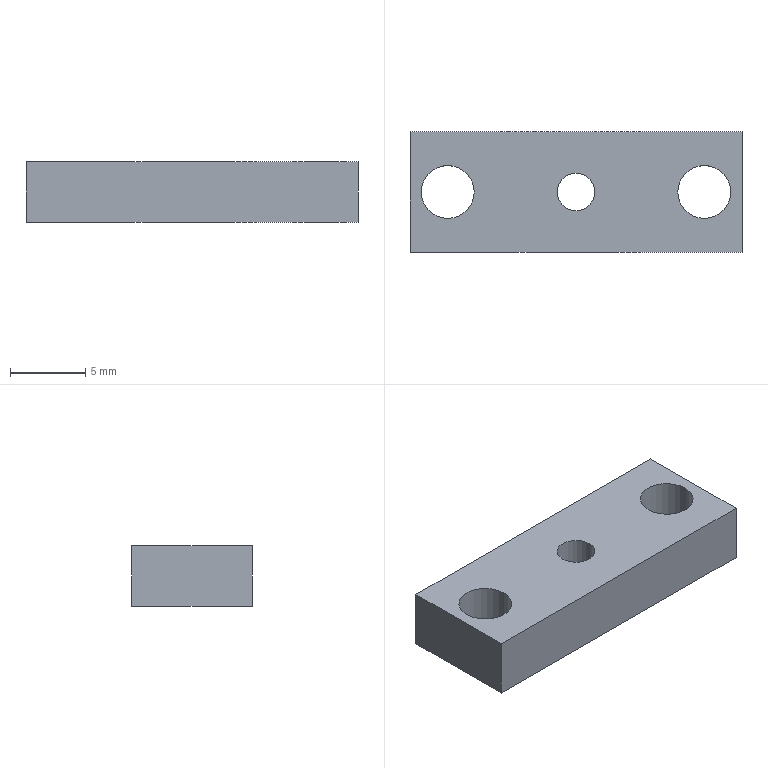Part | STEP file | X77b-01015 | 1 solid | 12 faces | box 22 x 8 x 4 mm | volume 607.396 mm3 | cylinder 6 | plane 6 | commonest cylinder face diameters 3.5 x4 2.5 x2
STEP:
#1=CARTESIAN_POINT('',(-1.25,-111.538,0.));
#2=VERTEX_POINT('',#1);
#3=CARTESIAN_POINT('',(1.25,-111.538,0.));
#4=VERTEX_POINT('',#3);
#5=CARTESIAN_POINT('',(0.,-111.538,0.));
#6=DIRECTION('',(0.,0.,1.));
#7=DIRECTION('',(1.,0.,0.));
#8=AXIS2_PLACEMENT_3D('',#5,#6,#7);
#9=CIRCLE('',#8,1.25);
#10=EDGE_CURVE('',#2,#4,#9,.T.);
#11=ORIENTED_EDGE('',*,*,#10,.F.);
#12=CARTESIAN_POINT('',(-1.25,-111.538,4.));
#13=VERTEX_POINT('',#12);
#14=CARTESIAN_POINT('',(-1.25,-111.538,4.));
#15=DIRECTION('',(0.,0.,1.));
#16=VECTOR('',#15,1000.);
#17=LINE('',#14,#16);
#18=EDGE_CURVE('',#2,#13,#17,.T.);
#19=ORIENTED_EDGE('',*,*,#18,.T.);
#20=CARTESIAN_POINT('',(1.25,-111.538,4.));
#21=VERTEX_POINT('',#20);
#22=CARTESIAN_POINT('',(0.,-111.538,4.));
#23=DIRECTION('',(0.,0.,1.));
#24=DIRECTION('',(1.,0.,0.));
#25=AXIS2_PLACEMENT_3D('',#22,#23,#24);
#26=CIRCLE('',#25,1.25);
#27=EDGE_CURVE('',#13,#21,#26,.T.);
#28=ORIENTED_EDGE('',*,*,#27,.T.);
#29=CARTESIAN_POINT('',(1.25,-111.538,4.));
#30=DIRECTION('',(0.,0.,1.));
#31=VECTOR('',#30,1000.);
#32=LINE('',#29,#31);
#33=EDGE_CURVE('',#4,#21,#32,.T.);
#34=ORIENTED_EDGE('',*,*,#33,.F.);
#35=EDGE_LOOP('',(#11,#19,#28,#34));
#36=FACE_OUTER_BOUND('',#35,.T.);
#37=CARTESIAN_POINT('',(0.,-111.538,4.));
#38=DIRECTION('',(0.,0.,1.));
#39=DIRECTION('',(1.,0.,0.));
#40=AXIS2_PLACEMENT_3D('',#37,#38,#39);
#41=CYLINDRICAL_SURFACE('',#40,1.25);
#42=ADVANCED_FACE('',(#36),#41,.F.);
#43=CARTESIAN_POINT('',(6.75,-111.538,4.));
#44=VERTEX_POINT('',#43);
#45=CARTESIAN_POINT('',(10.25,-111.538,4.));
#46=VERTEX_POINT('',#45);
#47=CARTESIAN_POINT('',(8.5,-111.538,4.));
#48=DIRECTION('',(0.,0.,1.));
#49=DIRECTION('',(1.,0.,0.));
#50=AXIS2_PLACEMENT_3D('',#47,#48,#49);
#51=CIRCLE('',#50,1.75);
#52=EDGE_CURVE('',#44,#46,#51,.T.);
#53=ORIENTED_EDGE('',*,*,#52,.T.);
#54=CARTESIAN_POINT('',(10.25,-111.538,0.));
#55=VERTEX_POINT('',#54);
#56=CARTESIAN_POINT('',(10.25,-111.538,4.));
#57=DIRECTION('',(0.,0.,-1.));
#58=VECTOR('',#57,1000.);
#59=LINE('',#56,#58);
#60=EDGE_CURVE('',#46,#55,#59,.T.);
#61=ORIENTED_EDGE('',*,*,#60,.T.);
#62=CARTESIAN_POINT('',(6.75,-111.538,0.));
#63=VERTEX_POINT('',#62);
#64=CARTESIAN_POINT('',(8.5,-111.538,0.));
#65=DIRECTION('',(0.,0.,1.));
#66=DIRECTION('',(1.,0.,0.));
#67=AXIS2_PLACEMENT_3D('',#64,#65,#66);
#68=CIRCLE('',#67,1.75);
#69=EDGE_CURVE('',#63,#55,#68,.T.);
#70=ORIENTED_EDGE('',*,*,#69,.F.);
#71=CARTESIAN_POINT('',(6.75,-111.538,4.));
#72=DIRECTION('',(0.,0.,-1.));
#73=VECTOR('',#72,1000.);
#74=LINE('',#71,#73);
#75=EDGE_CURVE('',#44,#63,#74,.T.);
#76=ORIENTED_EDGE('',*,*,#75,.F.);
#77=EDGE_LOOP('',(#53,#61,#70,#76));
#78=FACE_OUTER_BOUND('',#77,.T.);
#79=CARTESIAN_POINT('',(8.5,-111.538,4.));
#80=DIRECTION('',(0.,0.,-1.));
#81=DIRECTION('',(-1.,0.,0.));
#82=AXIS2_PLACEMENT_3D('',#79,#80,#81);
#83=CYLINDRICAL_SURFACE('',#82,1.75);
#84=ADVANCED_FACE('',(#78),#83,.F.);
#85=CARTESIAN_POINT('',(-10.25,-111.538,4.));
#86=VERTEX_POINT('',#85);
#87=CARTESIAN_POINT('',(-6.75,-111.538,4.));
#88=VERTEX_POINT('',#87);
#89=CARTESIAN_POINT('',(-8.5,-111.538,4.));
#90=DIRECTION('',(0.,0.,1.));
#91=DIRECTION('',(1.,0.,0.));
#92=AXIS2_PLACEMENT_3D('',#89,#90,#91);
#93=CIRCLE('',#92,1.75);
#94=EDGE_CURVE('',#86,#88,#93,.T.);
#95=ORIENTED_EDGE('',*,*,#94,.T.);
#96=CARTESIAN_POINT('',(-6.75,-111.538,0.));
#97=VERTEX_POINT('',#96);
#98=CARTESIAN_POINT('',(-6.75,-111.538,4.));
#99=DIRECTION('',(0.,0.,-1.));
#100=VECTOR('',#99,1000.);
#101=LINE('',#98,#100);
#102=EDGE_CURVE('',#88,#97,#101,.T.);
#103=ORIENTED_EDGE('',*,*,#102,.T.);
#104=CARTESIAN_POINT('',(-10.25,-111.538,0.));
#105=VERTEX_POINT('',#104);
#106=CARTESIAN_POINT('',(-8.5,-111.538,0.));
#107=DIRECTION('',(0.,0.,1.));
#108=DIRECTION('',(1.,0.,0.));
#109=AXIS2_PLACEMENT_3D('',#106,#107,#108);
#110=CIRCLE('',#109,1.75);
#111=EDGE_CURVE('',#105,#97,#110,.T.);
#112=ORIENTED_EDGE('',*,*,#111,.F.);
#113=CARTESIAN_POINT('',(-10.25,-111.538,4.));
#114=DIRECTION('',(0.,0.,-1.));
#115=VECTOR('',#114,1000.);
#116=LINE('',#113,#115);
#117=EDGE_CURVE('',#86,#105,#116,.T.);
#118=ORIENTED_EDGE('',*,*,#117,.F.);
#119=EDGE_LOOP('',(#95,#103,#112,#118));
#120=FACE_OUTER_BOUND('',#119,.T.);
#121=CARTESIAN_POINT('',(-8.5,-111.538,4.));
#122=DIRECTION('',(0.,0.,-1.));
#123=DIRECTION('',(-1.,0.,0.));
#124=AXIS2_PLACEMENT_3D('',#121,#122,#123);
#125=CYLINDRICAL_SURFACE('',#124,1.75);
#126=ADVANCED_FACE('',(#120),#125,.F.);
#127=CARTESIAN_POINT('',(0.,-111.538,4.));
#128=DIRECTION('',(0.,0.,1.));
#129=DIRECTION('',(1.,0.,0.));
#130=AXIS2_PLACEMENT_3D('',#127,#128,#129);
#131=CIRCLE('',#130,1.25);
#132=EDGE_CURVE('',#21,#13,#131,.T.);
#133=ORIENTED_EDGE('',*,*,#132,.F.);
#134=ORIENTED_EDGE('',*,*,#27,.F.);
#135=EDGE_LOOP('',(#133,#134));
#136=FACE_BOUND('',#135,.T.);
#137=ORIENTED_EDGE('',*,*,#94,.F.);
#138=CARTESIAN_POINT('',(-8.5,-111.538,4.));
#139=DIRECTION('',(0.,0.,1.));
#140=DIRECTION('',(1.,0.,0.));
#141=AXIS2_PLACEMENT_3D('',#138,#139,#140);
#142=CIRCLE('',#141,1.75);
#143=EDGE_CURVE('',#88,#86,#142,.T.);
#144=ORIENTED_EDGE('',*,*,#143,.F.);
#145=EDGE_LOOP('',(#137,#144));
#146=FACE_BOUND('',#145,.T.);
#147=CARTESIAN_POINT('',(-11.,-107.538,4.));
#148=VERTEX_POINT('',#147);
#149=CARTESIAN_POINT('',(-11.,-115.538,4.));
#150=VERTEX_POINT('',#149);
#151=CARTESIAN_POINT('',(-11.,-107.538,4.));
#152=DIRECTION('',(0.,-1.,0.));
#153=VECTOR('',#152,1000.);
#154=LINE('',#151,#153);
#155=EDGE_CURVE('',#148,#150,#154,.T.);
#156=ORIENTED_EDGE('',*,*,#155,.T.);
#157=CARTESIAN_POINT('',(11.,-115.538,4.));
#158=VERTEX_POINT('',#157);
#159=CARTESIAN_POINT('',(-11.,-115.538,4.));
#160=DIRECTION('',(1.,0.,0.));
#161=VECTOR('',#160,1000.);
#162=LINE('',#159,#161);
#163=EDGE_CURVE('',#150,#158,#162,.T.);
#164=ORIENTED_EDGE('',*,*,#163,.T.);
#165=CARTESIAN_POINT('',(11.,-107.538,4.));
#166=VERTEX_POINT('',#165);
#167=CARTESIAN_POINT('',(11.,-107.538,4.));
#168=DIRECTION('',(0.,1.,0.));
#169=VECTOR('',#168,1000.);
#170=LINE('',#167,#169);
#171=EDGE_CURVE('',#158,#166,#170,.T.);
#172=ORIENTED_EDGE('',*,*,#171,.T.);
#173=CARTESIAN_POINT('',(-11.,-107.538,4.));
#174=DIRECTION('',(-1.,0.,0.));
#175=VECTOR('',#174,1000.);
#176=LINE('',#173,#175);
#177=EDGE_CURVE('',#166,#148,#176,.T.);
#178=ORIENTED_EDGE('',*,*,#177,.T.);
#179=EDGE_LOOP('',(#156,#164,#172,#178));
#180=FACE_OUTER_BOUND('',#179,.T.);
#181=ORIENTED_EDGE('',*,*,#52,.F.);
#182=CARTESIAN_POINT('',(8.5,-111.538,4.));
#183=DIRECTION('',(0.,0.,1.));
#184=DIRECTION('',(1.,0.,0.));
#185=AXIS2_PLACEMENT_3D('',#182,#183,#184);
#186=CIRCLE('',#185,1.75);
#187=EDGE_CURVE('',#46,#44,#186,.T.);
#188=ORIENTED_EDGE('',*,*,#187,.F.);
#189=EDGE_LOOP('',(#181,#188));
#190=FACE_BOUND('',#189,.T.);
#191=CARTESIAN_POINT('',(-11.,-115.538,4.));
#192=DIRECTION('',(0.,0.,1.));
#193=DIRECTION('',(1.,0.,0.));
#194=AXIS2_PLACEMENT_3D('',#191,#192,#193);
#195=PLANE('',#194);
#196=ADVANCED_FACE('',(#136,#146,#180,#190),#195,.T.);
#197=CARTESIAN_POINT('',(0.,-111.538,0.));
#198=DIRECTION('',(0.,0.,1.));
#199=DIRECTION('',(1.,0.,0.));
#200=AXIS2_PLACEMENT_3D('',#197,#198,#199);
#201=CIRCLE('',#200,1.25);
#202=EDGE_CURVE('',#4,#2,#201,.T.);
#203=ORIENTED_EDGE('',*,*,#202,.T.);
#204=ORIENTED_EDGE('',*,*,#10,.T.);
#205=EDGE_LOOP('',(#203,#204));
#206=FACE_BOUND('',#205,.T.);
#207=ORIENTED_EDGE('',*,*,#111,.T.);
#208=CARTESIAN_POINT('',(-8.5,-111.538,0.));
#209=DIRECTION('',(0.,0.,1.));
#210=DIRECTION('',(1.,0.,0.));
#211=AXIS2_PLACEMENT_3D('',#208,#209,#210);
#212=CIRCLE('',#211,1.75);
#213=EDGE_CURVE('',#97,#105,#212,.T.);
#214=ORIENTED_EDGE('',*,*,#213,.T.);
#215=EDGE_LOOP('',(#207,#214));
#216=FACE_BOUND('',#215,.T.);
#217=CARTESIAN_POINT('',(-11.,-107.538,0.));
#218=VERTEX_POINT('',#217);
#219=CARTESIAN_POINT('',(-11.,-115.538,0.));
#220=VERTEX_POINT('',#219);
#221=CARTESIAN_POINT('',(-11.,-107.538,0.));
#222=DIRECTION('',(0.,-1.,0.));
#223=VECTOR('',#222,1000.);
#224=LINE('',#221,#223);
#225=EDGE_CURVE('',#218,#220,#224,.T.);
#226=ORIENTED_EDGE('',*,*,#225,.F.);
#227=CARTESIAN_POINT('',(11.,-107.538,0.));
#228=VERTEX_POINT('',#227);
#229=CARTESIAN_POINT('',(-11.,-107.538,0.));
#230=DIRECTION('',(-1.,0.,0.));
#231=VECTOR('',#230,1000.);
#232=LINE('',#229,#231);
#233=EDGE_CURVE('',#228,#218,#232,.T.);
#234=ORIENTED_EDGE('',*,*,#233,.F.);
#235=CARTESIAN_POINT('',(11.,-115.538,0.));
#236=VERTEX_POINT('',#235);
#237=CARTESIAN_POINT('',(11.,-107.538,0.));
#238=DIRECTION('',(0.,1.,0.));
#239=VECTOR('',#238,1000.);
#240=LINE('',#237,#239);
#241=EDGE_CURVE('',#236,#228,#240,.T.);
#242=ORIENTED_EDGE('',*,*,#241,.F.);
#243=CARTESIAN_POINT('',(-11.,-115.538,0.));
#244=DIRECTION('',(1.,0.,0.));
#245=VECTOR('',#244,1000.);
#246=LINE('',#243,#245);
#247=EDGE_CURVE('',#220,#236,#246,.T.);
#248=ORIENTED_EDGE('',*,*,#247,.F.);
#249=EDGE_LOOP('',(#226,#234,#242,#248));
#250=FACE_OUTER_BOUND('',#249,.T.);
#251=ORIENTED_EDGE('',*,*,#69,.T.);
#252=CARTESIAN_POINT('',(8.5,-111.538,0.));
#253=DIRECTION('',(0.,0.,1.));
#254=DIRECTION('',(1.,0.,0.));
#255=AXIS2_PLACEMENT_3D('',#252,#253,#254);
#256=CIRCLE('',#255,1.75);
#257=EDGE_CURVE('',#55,#63,#256,.T.);
#258=ORIENTED_EDGE('',*,*,#257,.T.);
#259=EDGE_LOOP('',(#251,#258));
#260=FACE_BOUND('',#259,.T.);
#261=CARTESIAN_POINT('',(-11.,-115.538,0.));
#262=DIRECTION('',(0.,0.,1.));
#263=DIRECTION('',(1.,0.,0.));
#264=AXIS2_PLACEMENT_3D('',#261,#262,#263);
#265=PLANE('',#264);
#266=ADVANCED_FACE('',(#206,#216,#250,#260),#265,.F.);
#267=ORIENTED_EDGE('',*,*,#225,.T.);
#268=CARTESIAN_POINT('',(-11.,-115.538,4.));
#269=DIRECTION('',(0.,0.,-1.));
#270=VECTOR('',#269,1000.);
#271=LINE('',#268,#270);
#272=EDGE_CURVE('',#150,#220,#271,.T.);
#273=ORIENTED_EDGE('',*,*,#272,.F.);
#274=ORIENTED_EDGE('',*,*,#155,.F.);
#275=CARTESIAN_POINT('',(-11.,-107.538,4.));
#276=DIRECTION('',(0.,0.,-1.));
#277=VECTOR('',#276,1000.);
#278=LINE('',#275,#277);
#279=EDGE_CURVE('',#148,#218,#278,.T.);
#280=ORIENTED_EDGE('',*,*,#279,.T.);
#281=EDGE_LOOP('',(#267,#273,#274,#280));
#282=FACE_OUTER_BOUND('',#281,.T.);
#283=CARTESIAN_POINT('',(-11.,-107.538,4.));
#284=DIRECTION('',(1.,0.,0.));
#285=DIRECTION('',(0.,1.,0.));
#286=AXIS2_PLACEMENT_3D('',#283,#284,#285);
#287=PLANE('',#286);
#288=ADVANCED_FACE('',(#282),#287,.F.);
#289=ORIENTED_EDGE('',*,*,#247,.T.);
#290=CARTESIAN_POINT('',(11.,-115.538,4.));
#291=DIRECTION('',(0.,0.,-1.));
#292=VECTOR('',#291,1000.);
#293=LINE('',#290,#292);
#294=EDGE_CURVE('',#158,#236,#293,.T.);
#295=ORIENTED_EDGE('',*,*,#294,.F.);
#296=ORIENTED_EDGE('',*,*,#163,.F.);
#297=ORIENTED_EDGE('',*,*,#272,.T.);
#298=EDGE_LOOP('',(#289,#295,#296,#297));
#299=FACE_OUTER_BOUND('',#298,.T.);
#300=CARTESIAN_POINT('',(-11.,-115.538,4.));
#301=DIRECTION('',(0.,1.,0.));
#302=DIRECTION('',(0.,0.,1.));
#303=AXIS2_PLACEMENT_3D('',#300,#301,#302);
#304=PLANE('',#303);
#305=ADVANCED_FACE('',(#299),#304,.F.);
#306=ORIENTED_EDGE('',*,*,#241,.T.);
#307=CARTESIAN_POINT('',(11.,-107.538,4.));
#308=DIRECTION('',(0.,0.,-1.));
#309=VECTOR('',#308,1000.);
#310=LINE('',#307,#309);
#311=EDGE_CURVE('',#166,#228,#310,.T.);
#312=ORIENTED_EDGE('',*,*,#311,.F.);
#313=ORIENTED_EDGE('',*,*,#171,.F.);
#314=ORIENTED_EDGE('',*,*,#294,.T.);
#315=EDGE_LOOP('',(#306,#312,#313,#314));
#316=FACE_OUTER_BOUND('',#315,.T.);
#317=CARTESIAN_POINT('',(11.,-107.538,4.));
#318=DIRECTION('',(-1.,0.,0.));
#319=DIRECTION('',(0.,-1.,0.));
#320=AXIS2_PLACEMENT_3D('',#317,#318,#319);
#321=PLANE('',#320);
#322=ADVANCED_FACE('',(#316),#321,.F.);
#323=ORIENTED_EDGE('',*,*,#233,.T.);
#324=ORIENTED_EDGE('',*,*,#279,.F.);
#325=ORIENTED_EDGE('',*,*,#177,.F.);
#326=ORIENTED_EDGE('',*,*,#311,.T.);
#327=EDGE_LOOP('',(#323,#324,#325,#326));
#328=FACE_OUTER_BOUND('',#327,.T.);
#329=CARTESIAN_POINT('',(-11.,-107.538,4.));
#330=DIRECTION('',(0.,-1.,0.));
#331=DIRECTION('',(0.,0.,-1.));
#332=AXIS2_PLACEMENT_3D('',#329,#330,#331);
#333=PLANE('',#332);
#334=ADVANCED_FACE('',(#328),#333,.F.);
#335=ORIENTED_EDGE('',*,*,#102,.F.);
#336=ORIENTED_EDGE('',*,*,#143,.T.);
#337=ORIENTED_EDGE('',*,*,#117,.T.);
#338=ORIENTED_EDGE('',*,*,#213,.F.);
#339=EDGE_LOOP('',(#335,#336,#337,#338));
#340=FACE_OUTER_BOUND('',#339,.T.);
#341=CARTESIAN_POINT('',(-8.5,-111.538,4.));
#342=DIRECTION('',(0.,0.,-1.));
#343=DIRECTION('',(-1.,0.,0.));
#344=AXIS2_PLACEMENT_3D('',#341,#342,#343);
#345=CYLINDRICAL_SURFACE('',#344,1.75);
#346=ADVANCED_FACE('',(#340),#345,.F.);
#347=ORIENTED_EDGE('',*,*,#60,.F.);
#348=ORIENTED_EDGE('',*,*,#187,.T.);
#349=ORIENTED_EDGE('',*,*,#75,.T.);
#350=ORIENTED_EDGE('',*,*,#257,.F.);
#351=EDGE_LOOP('',(#347,#348,#349,#350));
#352=FACE_OUTER_BOUND('',#351,.T.);
#353=CARTESIAN_POINT('',(8.5,-111.538,4.));
#354=DIRECTION('',(0.,0.,-1.));
#355=DIRECTION('',(-1.,0.,0.));
#356=AXIS2_PLACEMENT_3D('',#353,#354,#355);
#357=CYLINDRICAL_SURFACE('',#356,1.75);
#358=ADVANCED_FACE('',(#352),#357,.F.);
#359=ORIENTED_EDGE('',*,*,#18,.F.);
#360=ORIENTED_EDGE('',*,*,#202,.F.);
#361=ORIENTED_EDGE('',*,*,#33,.T.);
#362=ORIENTED_EDGE('',*,*,#132,.T.);
#363=EDGE_LOOP('',(#359,#360,#361,#362));
#364=FACE_OUTER_BOUND('',#363,.T.);
#365=CARTESIAN_POINT('',(0.,-111.538,4.));
#366=DIRECTION('',(0.,0.,1.));
#367=DIRECTION('',(1.,0.,0.));
#368=AXIS2_PLACEMENT_3D('',#365,#366,#367);
#369=CYLINDRICAL_SURFACE('',#368,1.25);
#370=ADVANCED_FACE('',(#364),#369,.F.);
#371=CLOSED_SHELL('',(#42,#84,#126,#196,#266,#288,#305,#322,#334,#346,#358,#370));
#372=MANIFOLD_SOLID_BREP('',#371);
#373=CARTESIAN_POINT('',(0.,0.,0.));
#374=DIRECTION('',(0.,0.,1.));
#375=DIRECTION('',(1.,0.,0.));
#376=AXIS2_PLACEMENT_3D('',#373,#374,#375);
#377=(LENGTH_UNIT()NAMED_UNIT(*)SI_UNIT(.MILLI.,.METRE.));
#378=UNCERTAINTY_MEASURE_WITH_UNIT(LENGTH_MEASURE(0.00001),#377,'','');
#379=(NAMED_UNIT(*)PLANE_ANGLE_UNIT()SI_UNIT($,.RADIAN.));
#380=(NAMED_UNIT(*)SI_UNIT($,.STERADIAN.)SOLID_ANGLE_UNIT());
#381=(GEOMETRIC_REPRESENTATION_CONTEXT(3)GLOBAL_UNCERTAINTY_ASSIGNED_CONTEXT((#378))GLOBAL_UNIT_ASSIGNED_CONTEXT((#377,#379,#380))REPRESENTATION_CONTEXT('',''));
#382=ADVANCED_BREP_SHAPE_REPRESENTATION('',(#372,#376),#381);